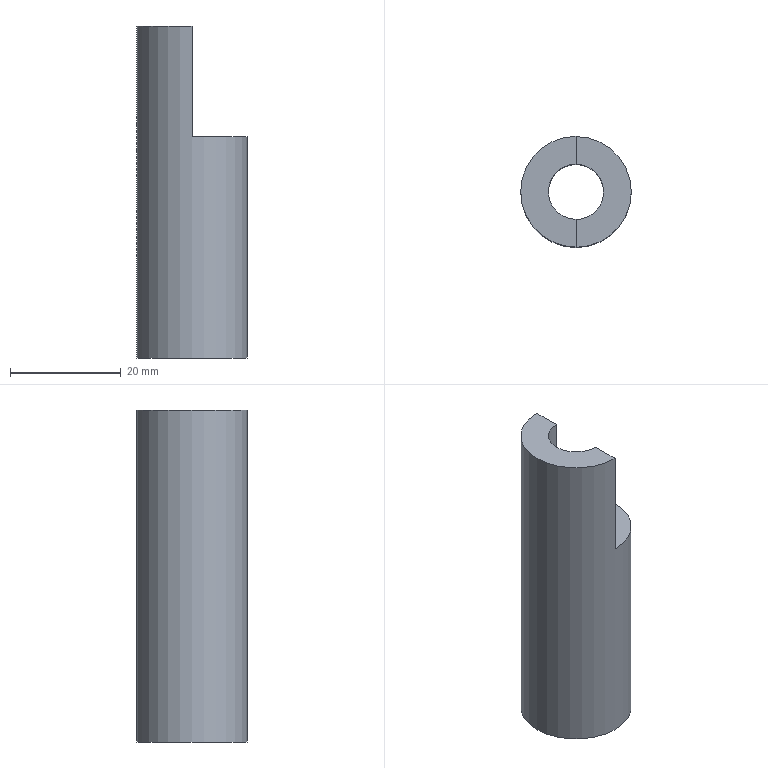Part | NX | features TH 2 | 1 solid | 7 faces | box 20 x 20 x 60 mm | volume 11781 mm3 | plane 5 | cylinder 2 | commonest cylinder face diameters 10 x1 20 x1
STEP:
#1=CARTESIAN_POINT('',(3252.,120.,-73.));
#2=VERTEX_POINT('',#1);
#3=CARTESIAN_POINT('',(3252.,120.,-93.));
#4=VERTEX_POINT('',#3);
#5=CARTESIAN_POINT('',(3252.,120.,-73.));
#6=DIRECTION('',(0.,0.,-1.));
#7=VECTOR('',#6,1000.);
#8=LINE('',#5,#7);
#9=EDGE_CURVE('',#2,#4,#8,.T.);
#10=ORIENTED_EDGE('',*,*,#9,.T.);
#11=CARTESIAN_POINT('',(3252.,125.,-93.));
#12=VERTEX_POINT('',#11);
#13=CARTESIAN_POINT('',(3252.,-193.,-93.));
#14=DIRECTION('',(0.,-1.,0.));
#15=VECTOR('',#14,1000.);
#16=LINE('',#13,#15);
#17=EDGE_CURVE('',#12,#4,#16,.T.);
#18=ORIENTED_EDGE('',*,*,#17,.F.);
#19=CARTESIAN_POINT('',(3252.,125.,-73.));
#20=VERTEX_POINT('',#19);
#21=CARTESIAN_POINT('',(3252.,125.,-83.));
#22=DIRECTION('',(0.,0.,1.));
#23=VECTOR('',#22,1000.);
#24=LINE('',#21,#23);
#25=EDGE_CURVE('',#12,#20,#24,.T.);
#26=ORIENTED_EDGE('',*,*,#25,.T.);
#27=CARTESIAN_POINT('',(3252.,-193.,-73.));
#28=DIRECTION('',(0.,-1.,0.));
#29=VECTOR('',#28,1000.);
#30=LINE('',#27,#29);
#31=EDGE_CURVE('',#20,#2,#30,.T.);
#32=ORIENTED_EDGE('',*,*,#31,.T.);
#33=EDGE_LOOP('',(#10,#18,#26,#32));
#34=FACE_BOUND('',#33,.T.);
#35=CARTESIAN_POINT('',(3252.,115.,-73.));
#36=DIRECTION('',(1.,0.,0.));
#37=DIRECTION('',(0.,0.,1.));
#38=AXIS2_PLACEMENT_3D('',#35,#36,#37);
#39=PLANE('',#38);
#40=ADVANCED_FACE('',(#34),#39,.T.);
#41=CARTESIAN_POINT('',(3242.,115.,-133.));
#42=VERTEX_POINT('',#41);
#43=CARTESIAN_POINT('',(3252.,115.,-133.));
#44=DIRECTION('',(0.,0.,1.));
#45=DIRECTION('',(-1.,0.,0.));
#46=AXIS2_PLACEMENT_3D('',#43,#44,#45);
#47=CIRCLE('',#46,10.);
#48=EDGE_CURVE('',#42,#42,#47,.T.);
#49=ORIENTED_EDGE('',*,*,#48,.T.);
#50=EDGE_LOOP('',(#49));
#51=FACE_BOUND('',#50,.T.);
#52=CARTESIAN_POINT('',(3252.,105.,-93.));
#53=VERTEX_POINT('',#52);
#54=CARTESIAN_POINT('',(3252.,115.,-93.));
#55=DIRECTION('',(0.,0.,1.));
#56=DIRECTION('',(-1.,0.,0.));
#57=AXIS2_PLACEMENT_3D('',#54,#55,#56);
#58=CIRCLE('',#57,10.);
#59=EDGE_CURVE('',#53,#12,#58,.T.);
#60=ORIENTED_EDGE('',*,*,#59,.F.);
#61=CARTESIAN_POINT('',(3252.,105.,-73.));
#62=VERTEX_POINT('',#61);
#63=CARTESIAN_POINT('',(3252.,105.,-83.));
#64=DIRECTION('',(0.,0.,-1.));
#65=VECTOR('',#64,1000.);
#66=LINE('',#63,#65);
#67=EDGE_CURVE('',#62,#53,#66,.T.);
#68=ORIENTED_EDGE('',*,*,#67,.F.);
#69=CARTESIAN_POINT('',(3252.,115.,-73.));
#70=DIRECTION('',(0.,0.,1.));
#71=DIRECTION('',(-1.,0.,0.));
#72=AXIS2_PLACEMENT_3D('',#69,#70,#71);
#73=CIRCLE('',#72,10.);
#74=EDGE_CURVE('',#20,#62,#73,.T.);
#75=ORIENTED_EDGE('',*,*,#74,.F.);
#76=ORIENTED_EDGE('',*,*,#25,.F.);
#77=EDGE_LOOP('',(#60,#68,#75,#76));
#78=FACE_BOUND('',#77,.T.);
#79=CARTESIAN_POINT('',(3252.,115.,-133.));
#80=DIRECTION('',(0.,0.,1.));
#81=DIRECTION('',(-1.,0.,0.));
#82=AXIS2_PLACEMENT_3D('',#79,#80,#81);
#83=CYLINDRICAL_SURFACE('',#82,10.);
#84=ADVANCED_FACE('',(#51,#78),#83,.T.);
#85=CARTESIAN_POINT('',(3247.,115.,-133.));
#86=VERTEX_POINT('',#85);
#87=CARTESIAN_POINT('',(3252.,115.,-133.));
#88=DIRECTION('',(0.,0.,-1.));
#89=DIRECTION('',(-1.,0.,0.));
#90=AXIS2_PLACEMENT_3D('',#87,#88,#89);
#91=CIRCLE('',#90,5.);
#92=EDGE_CURVE('',#86,#86,#91,.T.);
#93=ORIENTED_EDGE('',*,*,#92,.F.);
#94=EDGE_LOOP('',(#93));
#95=FACE_BOUND('',#94,.T.);
#96=ORIENTED_EDGE('',*,*,#48,.F.);
#97=EDGE_LOOP('',(#96));
#98=FACE_BOUND('',#97,.T.);
#99=CARTESIAN_POINT('',(1598.5,-193.,-133.));
#100=DIRECTION('',(0.,0.,-1.));
#101=DIRECTION('',(-1.,0.,0.));
#102=AXIS2_PLACEMENT_3D('',#99,#100,#101);
#103=PLANE('',#102);
#104=ADVANCED_FACE('',(#95,#98),#103,.T.);
#105=CARTESIAN_POINT('',(3252.,110.,-93.));
#106=VERTEX_POINT('',#105);
#107=CARTESIAN_POINT('',(3252.,115.,-93.));
#108=DIRECTION('',(0.,0.,-1.));
#109=DIRECTION('',(-1.,0.,0.));
#110=AXIS2_PLACEMENT_3D('',#107,#108,#109);
#111=CIRCLE('',#110,5.);
#112=EDGE_CURVE('',#4,#106,#111,.T.);
#113=ORIENTED_EDGE('',*,*,#112,.T.);
#114=CARTESIAN_POINT('',(3252.,-193.,-93.));
#115=DIRECTION('',(0.,-1.,0.));
#116=VECTOR('',#115,1000.);
#117=LINE('',#114,#116);
#118=EDGE_CURVE('',#106,#53,#117,.T.);
#119=ORIENTED_EDGE('',*,*,#118,.T.);
#120=ORIENTED_EDGE('',*,*,#59,.T.);
#121=ORIENTED_EDGE('',*,*,#17,.T.);
#122=EDGE_LOOP('',(#113,#119,#120,#121));
#123=FACE_BOUND('',#122,.T.);
#124=CARTESIAN_POINT('',(1598.5,-193.,-93.));
#125=DIRECTION('',(0.,0.,-1.));
#126=DIRECTION('',(-1.,0.,0.));
#127=AXIS2_PLACEMENT_3D('',#124,#125,#126);
#128=PLANE('',#127);
#129=ADVANCED_FACE('',(#123),#128,.F.);
#130=CARTESIAN_POINT('',(3252.,110.,-73.));
#131=VERTEX_POINT('',#130);
#132=CARTESIAN_POINT('',(3252.,110.,-73.));
#133=DIRECTION('',(0.,0.,1.));
#134=VECTOR('',#133,1000.);
#135=LINE('',#132,#134);
#136=EDGE_CURVE('',#106,#131,#135,.T.);
#137=ORIENTED_EDGE('',*,*,#136,.T.);
#138=CARTESIAN_POINT('',(3252.,-193.,-73.));
#139=DIRECTION('',(0.,-1.,0.));
#140=VECTOR('',#139,1000.);
#141=LINE('',#138,#140);
#142=EDGE_CURVE('',#131,#62,#141,.T.);
#143=ORIENTED_EDGE('',*,*,#142,.T.);
#144=ORIENTED_EDGE('',*,*,#67,.T.);
#145=ORIENTED_EDGE('',*,*,#118,.F.);
#146=EDGE_LOOP('',(#137,#143,#144,#145));
#147=FACE_BOUND('',#146,.T.);
#148=CARTESIAN_POINT('',(3252.,115.,-73.));
#149=DIRECTION('',(1.,0.,0.));
#150=DIRECTION('',(0.,0.,1.));
#151=AXIS2_PLACEMENT_3D('',#148,#149,#150);
#152=PLANE('',#151);
#153=ADVANCED_FACE('',(#147),#152,.T.);
#154=CARTESIAN_POINT('',(3252.,115.,-73.));
#155=DIRECTION('',(0.,0.,1.));
#156=DIRECTION('',(-1.,0.,0.));
#157=AXIS2_PLACEMENT_3D('',#154,#155,#156);
#158=CIRCLE('',#157,5.);
#159=EDGE_CURVE('',#2,#131,#158,.T.);
#160=ORIENTED_EDGE('',*,*,#159,.F.);
#161=ORIENTED_EDGE('',*,*,#31,.F.);
#162=ORIENTED_EDGE('',*,*,#74,.T.);
#163=ORIENTED_EDGE('',*,*,#142,.F.);
#164=EDGE_LOOP('',(#160,#161,#162,#163));
#165=FACE_BOUND('',#164,.T.);
#166=CARTESIAN_POINT('',(1598.5,-193.,-73.));
#167=DIRECTION('',(0.,0.,-1.));
#168=DIRECTION('',(-1.,0.,0.));
#169=AXIS2_PLACEMENT_3D('',#166,#167,#168);
#170=PLANE('',#169);
#171=ADVANCED_FACE('',(#165),#170,.F.);
#172=ORIENTED_EDGE('',*,*,#9,.F.);
#173=ORIENTED_EDGE('',*,*,#159,.T.);
#174=ORIENTED_EDGE('',*,*,#136,.F.);
#175=ORIENTED_EDGE('',*,*,#112,.F.);
#176=EDGE_LOOP('',(#172,#173,#174,#175));
#177=FACE_BOUND('',#176,.T.);
#178=ORIENTED_EDGE('',*,*,#92,.T.);
#179=EDGE_LOOP('',(#178));
#180=FACE_BOUND('',#179,.T.);
#181=CARTESIAN_POINT('',(3252.,115.,-73.));
#182=DIRECTION('',(0.,0.,-1.));
#183=DIRECTION('',(1.,0.,0.));
#184=AXIS2_PLACEMENT_3D('',#181,#182,#183);
#185=CYLINDRICAL_SURFACE('',#184,5.);
#186=ADVANCED_FACE('',(#177,#180),#185,.F.);
#187=CLOSED_SHELL('',(#40,#84,#104,#129,#153,#171,#186));
#188=MANIFOLD_SOLID_BREP('',#187);
#189=(LENGTH_UNIT()NAMED_UNIT(*)SI_UNIT(.MILLI.,.METRE.));
#190=UNCERTAINTY_MEASURE_WITH_UNIT(LENGTH_MEASURE(0.00001),#189,'','');
#191=(NAMED_UNIT(*)PLANE_ANGLE_UNIT()SI_UNIT($,.RADIAN.));
#192=(NAMED_UNIT(*)SI_UNIT($,.STERADIAN.)SOLID_ANGLE_UNIT());
#193=(GEOMETRIC_REPRESENTATION_CONTEXT(3)GLOBAL_UNCERTAINTY_ASSIGNED_CONTEXT((#190))GLOBAL_UNIT_ASSIGNED_CONTEXT((#189,#191,#192))REPRESENTATION_CONTEXT('',''));
#194=ADVANCED_BREP_SHAPE_REPRESENTATION('',(#188),#193);